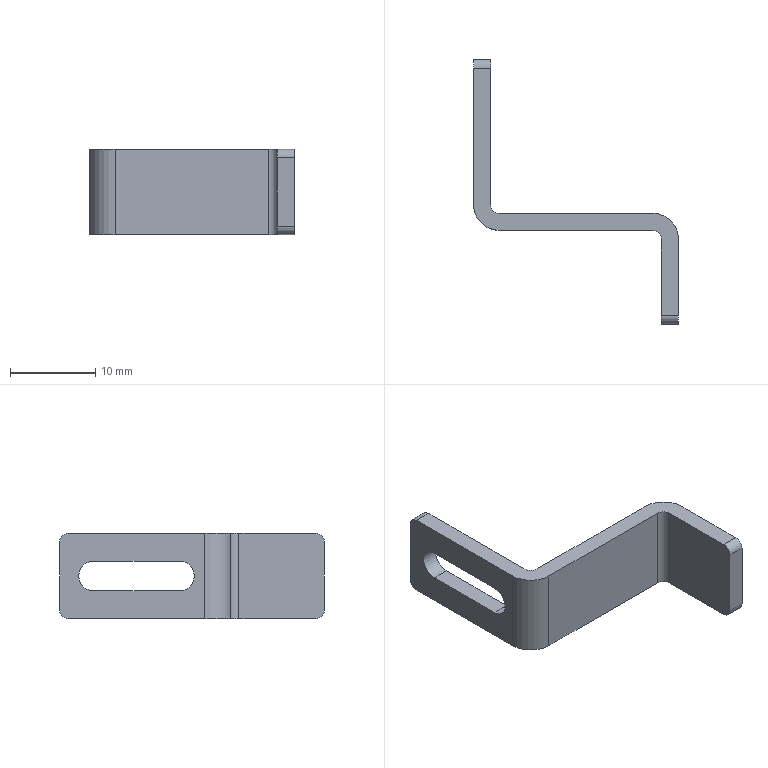Part | STEP file | 0-19-22 Sensor bracket | 1 solid | 22 faces | box 24 x 31 x 10 mm | volume 934.705 mm3 | plane 12 | cylinder 10 | commonest cylinder face diameters 2 x6 3.5 x2 6 x2